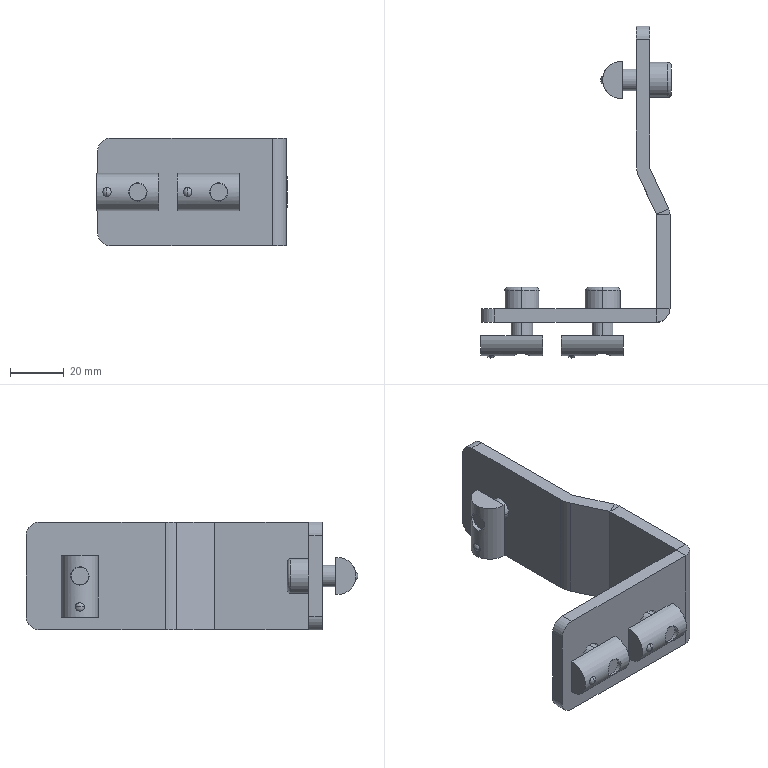Part | SolidWorks | features CompositeCurve 1 | 7 solids | 439 faces | box 70.833 x 123.25 x 40 mm | volume 44088 mm3 | plane 277 | spline 102 | cylinder 36 | cone 12 | torus 6 | sphere 6 | commonest cylinder face diameters 6.8 x6 8 x6 9 x6 13 x6 10 x4 13.848 x3